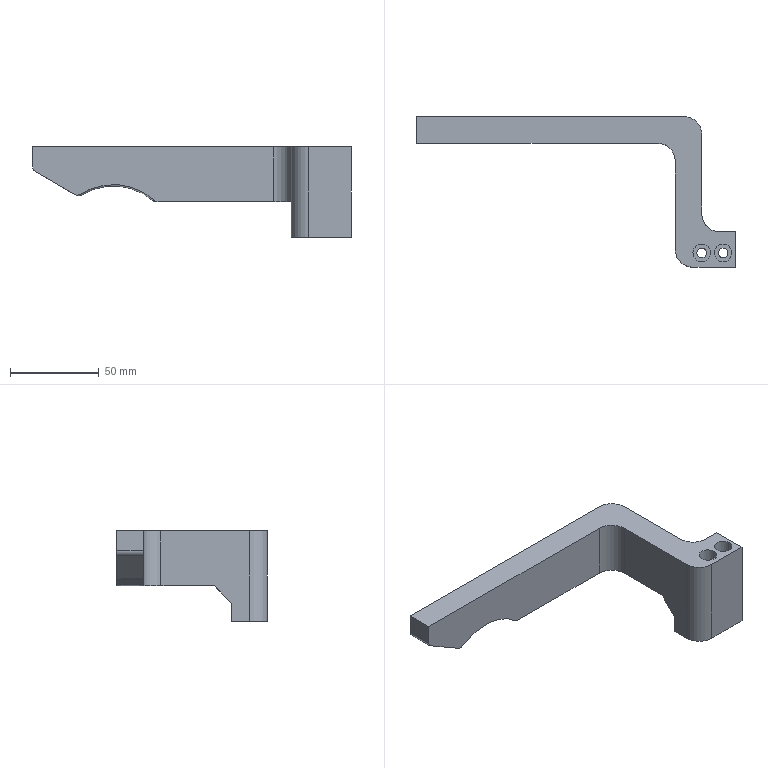NC program | NX | posted with a generic post | part box 180 x 85 x 51 mm
Lines 27156 to 29209 of 44959, first 1814 of 2034 lines:
(FLOOR_WALL_COPY , TOOL : D63)
N54298 T01 M6
N54300 G54
N54302 G17 G0 G90 X-129.5 Y-19. S6500 M3
N54304 G43 Z30. H1
N54306 Z3.
N54308 G94 G1 Z0. F1500.
N54310 X-121.503
N54312 X102.503
N54314 X105.503
N54316 Z3.
N54318 G0 Z30.
N54320 X-129.5
N54322 Z2.
N54324 G1 Z-1.
N54326 X-121.503
N54328 X102.503
N54330 X105.503
N54332 Z2.
N54334 G0 Z30.
N54336 X-129.5
N54338 Z1.
N54340 G1 Z-2.
N54342 X-121.503
N54344 X102.503
N54346 X105.503
N54348 Z1.
N54350 G0 Z30.
N54352 X-129.5
N54354 Z0.
N54356 G1 Z-3.
N54358 X-121.503
N54360 X102.503
N54362 X105.503
N54364 Z0.
N54366 G0 Z30.
N54368 X-129.5
N54370 Z-1.
N54372 G1 Z-4.
N54374 X-121.503
N54376 X102.503
N54378 X105.503
N54380 Z-1.
N54382 G0 Z30.
N54384 X-129.5
N54386 Z-2.
N54388 G1 Z-5.
N54390 X-121.503
N54392 X102.503
N54394 X105.503
N54396 Z-2.
N54398 G0 Z30.
N54400 X-129.5
N54402 Z-3.
N54404 G1 Z-6.
N54406 X-121.503
N54408 X102.503
N54410 X105.503
N54412 Z-3.
N54414 G0 Z30.
N54416 X-129.5
N54418 Z-4.
N54420 G1 Z-7.
N54422 X-121.503
N54424 X102.503
N54426 X105.503
N54428 Z-4.
N54430 G0 Z30.
N54432 X-129.5
N54434 Z-5.
N54436 G1 Z-8.
N54438 X-121.503
N54440 X102.503
N54442 X105.503
N54444 Z-5.
N54446 G0 Z30.
N54448 X-129.5
N54450 Z-6.
N54452 G1 Z-9.
N54454 X-121.503
N54456 X102.503
N54458 X105.503
N54460 Z-6.
N54462 G0 Z30.
N54464 X-129.5
N54466 Z-7.
N54468 G1 Z-10.
N54470 X-121.503
N54472 X102.503
N54474 X105.503
N54476 Z-7.
N54478 G0 Z30.
N54480 X-129.5
N54482 Z-8.
N54484 G1 Z-11.
N54486 X-121.503
N54488 X102.503
N54490 X105.503
N54492 Z-8.
N54494 G0 Z30.
N54496 X-129.5
N54498 Z-9.
N54500 G1 Z-12.
N54502 X-121.503
N54504 X102.503
N54506 X105.503
N54508 Z-9.
N54510 G0 Z30.
N54512 X-129.5
N54514 Z-10.
N54516 G1 Z-13.
N54518 X-121.503
N54520 X102.503
N54522 X105.503
N54524 Z-10.
N54526 G0 Z30.
N54528 X-129.5
N54530 Z-11.
N54532 G1 Z-14.
N54534 X-121.503
N54536 X102.503
N54538 X105.503
N54540 Z-11.
N54542 G0 Z30.
N54544 X-129.5
N54546 Z-12.
N54548 G1 Z-15.
N54550 X-121.503
N54552 X102.503
N54554 X105.503
N54556 Z-12.
N54558 G0 Z30.
N54560 X-129.5
N54562 Z-13.
N54564 G1 Z-16.
N54566 X-121.503
N54568 X102.503
N54570 X105.503
N54572 Z-13.
N54574 G0 Z30.
N54576 X-129.5
N54578 Z-14.
N54580 G1 Z-17.
N54582 X-121.503
N54584 X102.503
N54586 X105.503
N54588 Z-14.
N54590 G0 Z30.
N54592 X-129.5
N54594 Z-15.
N54596 G1 Z-18.
N54598 X-121.503
N54600 X102.503
N54602 X105.503
N54604 Z-15.
N54606 G0 Z30.
N54608 X-129.5
N54610 Z-16.
N54612 G1 Z-19.
N54614 X-121.503
N54616 X102.503
N54618 X105.503
N54620 Z-16.
N54622 G0 Z30.
N54624 X-129.5
N54626 Z-17.
N54628 G1 Z-20.
N54630 X-121.503
N54632 X102.503
N54634 X105.503
N54636 Z-17.
N54638 G0 Z30.
N54640 M5
(ZLEVEL_PROFILE , TOOL : D12C)
N54642 T12 M6
N54644 G54
N54646 G17 G0 G90 X98.933 Y13.081 S9500 M3
N54648 G43 Z30. H12
N54650 Z2.51
N54652 G94 G1 Z-0.49 F1000.
N54654 X97.362 Y15.801
N54656 G3 X96.323 Y16.401 R1.2
N54658 G1 X85.881 Y16.4 F2500.
N54660 X56.
N54662 X55.197 Y16.453
N54664 X55.137 Y16.4
N54666 X49.677 Y16.401
N54668 Z-0.98
N54670 X55.137 Y16.4
N54672 X55.197 Y16.453
N54674 X56. Y16.4
N54676 X85.881
N54678 X96.323 Y16.401
N54680 Z-1.47
N54682 X85.881 Y16.4
N54684 X56.
N54686 X55.197 Y16.453
N54688 X55.137 Y16.4
N54690 X49.677
N54692 Z-1.96
N54694 X55.137
N54696 X55.197 Y16.453
N54698 X56. Y16.4
N54700 X85.881
N54702 X96.323 Y16.401
N54704 Z-2.45
N54706 X85.881 Y16.4
N54708 X56.
N54710 X55.197 Y16.453
N54712 X55.137 Y16.4
N54714 X49.677
N54716 Z-2.94
N54718 X55.137
N54720 X55.197 Y16.453
N54722 X56. Y16.4
N54724 X85.881
N54726 X96.323 Y16.401
N54728 Z-3.43
N54730 X85.881 Y16.4
N54732 X56.
N54734 X55.197 Y16.453
N54736 X55.137 Y16.4
N54738 X49.677
N54740 Z-3.92
N54742 X55.137
N54744 X55.197 Y16.453
N54746 X56. Y16.4
N54748 X85.881
N54750 X96.323 Y16.401
N54752 Z-4.41
N54754 X85.881 Y16.4
N54756 X56.462
N54758 G2 X55.197 Y16.453 R9.583
N54760 G1 X55.137 Y16.4
N54762 X49.677
N54764 Z-4.9
N54766 X55.137
N54768 X55.197 Y16.453
N54770 G3 X56.462 Y16.4 R9.572
N54772 G1 X85.881
N54774 X96.323 Y16.401
N54776 Z-5.39
N54778 X85.881 Y16.4
N54780 X56.462
N54782 G2 X55.197 Y16.453 R9.562
N54784 G1 X55.137 Y16.4
N54786 X49.677
N54788 Z-5.88
N54790 X55.137
N54792 X55.197 Y16.453
N54794 G3 X56.462 Y16.4 R9.551
N54796 G1 X85.881
N54798 X96.323 Y16.401
N54800 Z-6.37
N54802 X85.881 Y16.4
N54804 X56.462
N54806 G2 X55.197 Y16.453 R9.54
N54808 G1 X55.137 Y16.4
N54810 X49.677
N54812 Z-6.86
N54814 X55.137
N54816 X55.197 Y16.453
N54818 G3 X56.462 Y16.4 R9.529
N54820 G1 X85.881
N54822 X96.323 Y16.401
N54824 Z-7.35
N54826 X85.881 Y16.4
N54828 X56.462
N54830 G2 X55.197 Y16.453 R9.518
N54832 G1 X55.137 Y16.4
N54834 X49.677
N54836 Z-7.84
N54838 X55.137
N54840 X55.197 Y16.453
N54842 G3 X56.462 Y16.4 R9.507
N54844 G1 X85.881
N54846 X96.323 Y16.401
N54848 Z-8.33
N54850 X85.881 Y16.4
N54852 X56.462
N54854 G2 X55.197 Y16.453 R9.497
N54856 G1 X55.137 Y16.4
N54858 X49.677
N54860 Z-8.82
N54862 X55.137
N54864 X55.197 Y16.453
N54866 G3 X56.462 Y16.4 R9.486
N54868 G1 X85.881
N54870 X96.323 Y16.401
N54872 Z-9.31
N54874 X85.881 Y16.4
N54876 X56.462
N54878 G2 X55.197 Y16.453 R9.475
N54880 G1 X55.137 Y16.4
N54882 X49.677
N54884 Z-9.8
N54886 X55.137
N54888 X55.197 Y16.453
N54890 G3 X56.462 Y16.4 R9.465
N54892 G1 X85.881
N54894 X96.323 Y16.401
N54896 G2 X97.362 Y15.801 R1.2
N54898 G1 X98.933 Y13.081
N54900 Z-6.8
N54902 G0 Z30.
(ZLEVEL_PROFILE_COPY , TOOL : D12C)
N54904 X87.319 Y12.8
N54906 Z-7.495
N54908 G1 Z-10.495 F1000.
N54910 X85.147 Y15.894
N54912 G3 X84.059 Y16.4 R1.2
N54914 X82.377 Y16.013 R6.277 F2500.
N54916 G1 X81.536 Y15.884
N54918 X77.7 Y15.864
N54920 X49.577
N54922 X49.512 Y15.867
N54924 X49.51 Y15.616 Z-10.743
N54926 X49.509 Y15.372 Z-10.99
N54928 X56. Y15.369
N54930 X81.101
N54932 G3 X84.182 Y16.235 R5.914
N54934 G1 X84.9 Y16.4
N54936 X85.741 Z-11.485
N54938 X84.937 Y16.235
N54940 G2 X81.271 Y14.884 R5.938
N54942 G1 X80.695 Y14.874
N54944 X49.577
N54946 X49.507 Y14.878
N54948 X49.506 Y14.626 Z-11.733
N54950 X49.504 Y14.383 Z-11.98
N54952 X49.577 Y14.379
N54954 X81.208
N54956 G3 X85.228 Y15.974 R5.862
N54958 G1 X85.505 Y16.235
N54960 X85.741 Y16.4
N54962 X86.582 Z-12.475
N54964 X86.023 Y16.235
N54966 G2 X81.312 Y13.889 R6.015
N54968 G1 X80.695 Y13.884
N54970 X49.577
N54972 X49.502 Y13.888
N54974 X49.501 Y13.636 Z-12.723
N54976 X49.5 Y13.393 Z-12.97
N54978 X49.577 Y13.389
N54980 X80.695
N54982 X81.317 Y13.392
N54984 G3 X86.582 Y16.4 R6.167
N54986 G1 X87.423 Z-13.465
N54988 X86.818 Y16.235
N54990 G2 X81.536 Y12.895 R6.072
N54992 G1 X73.375 Y12.894
N54994 X49.577
N54996 X49.498 Y12.898
N54998 Y12.646 Z-13.713
N55000 Y12.403 Z-13.96
N55002 X49.577 Y12.399
N55004 X72.978
N55006 X81.536
N55008 G3 X87.128 Y16.235 R6.086
N55010 G1 X87.423 Y16.4
N55012 X88.264 Z-14.455
N55014 X87.423 Y16.302
N55016 G2 X81.536 Y11.904 R6.089
N55018 G1 X49.577
N55020 X49.498 Y11.908
N55022 Y11.656 Z-14.703
N55024 Y11.413 Z-14.95
N55026 X49.577 Y11.409
N55028 X79.854
N55030 X80.302 Y11.422
N55032 X79.966 Y11.163 Z-15.198
N55034 X79.629 Y10.925 Z-15.445
N55036 X79.013 Y10.914
N55038 X49.577
N55040 X49.498 Y10.918
N55042 Y10.666 Z-15.693
N55044 Y10.423 Z-15.94
N55046 X49.577 Y10.419
N55048 X71.835
N55050 X79.139 Y10.426
N55052 X78.96 Y10.171 Z-16.188
N55054 X78.78 Y9.931 Z-16.435
N55056 X78.172 Y9.924
N55058 X49.577
N55060 X49.498 Y9.928
N55062 X49.499 Y9.676 Z-16.683
N55064 Y9.433 Z-16.93
N55066 X49.577 Y9.429
N55068 X78.172
N55070 X78.469 Y9.437
N55072 X78.356 Y9.181 Z-17.178
N55074 X78.243 Y8.938 Z-17.425
N55076 X78.172 Y8.934
N55078 X49.577
N55080 X49.502 Y8.938
N55082 X49.503 Y8.686 Z-17.673
N55084 X49.505 Y8.443 Z-17.92
N55086 X49.577 Y8.439
N55088 X71.208
N55090 X78.063 Y8.44
N55092 X77.991 Y8.191 Z-18.168
N55094 X77.92 Y7.948 Z-18.415
N55096 X71.444 Y7.944
N55098 X49.577
N55100 X49.507 Y7.948
N55102 X49.508 Y7.696 Z-18.663
N55104 X49.509 Y7.453 Z-18.91
N55106 X49.577 Y7.449
N55108 X71.058
N55110 X77.822 Y7.455
N55112 X77.782 Y7.201 Z-19.158
N55114 X77.743 Y6.956 Z-19.405
N55116 X71.019 Y6.954
N55118 X56.
N55120 X49.512 Y6.955
N55122 X49.513 Y6.706 Z-19.653
N55124 X49.514 Y6.47 Z-19.9
N55126 X56. Y6.466
N55128 X77.331
N55130 X77.691 Y6.474
N55132 G2 X78.744 Y5.898 R1.2
N55134 G1 X80.35 Y3.257
N55136 Z-16.9
N55138 G0 Z30.
(ZLEVEL_PROFILE_COPY_COPY_COPY , TOOL : D12C)
N55140 X-69.287 Y-51.578
N55142 Z-17.491
N55144 G1 Z-20.491 F1000.
N55146 X-66.638 Y-50.047
N55148 G3 X-66.039 Y-49.008 R1.2
N55150 G1 X-66.045 Y-37.949 F2500.
N55152 X-66.03 Y-37.719
N55154 G3 X-66.563 Y-36.644 R1.2
N55156 G1 X-69.324 Y-34.809
N55158 Z-17.491
N55160 G0 X-70.204 Y-19.451 Z-17.982
N55162 G1 Z-20.982 F1000.
N55164 X-67.458 Y-21.119
N55166 G2 X-66.881 Y-22.171 R1.2
N55168 G1 X-66.895 Y-22.783 F2500.
N55170 X-66.889 Y-49.013
N55172 X-67.32 Y-49.015 Z-21.227
N55174 X-67.739 Y-49.018 Z-21.472
N55176 Y-20.995
N55178 X-68.17 Y-20.992 Z-21.718
N55180 X-68.589 Y-20.99 Z-21.963
N55182 Y-49.023
N55184 X-69.02 Y-49.025 Z-22.209
N55186 X-69.439 Y-49.028 Z-22.454
N55188 Y-20.984
N55190 X-69.87 Y-20.981 Z-22.7
N55192 X-70.289 Y-20.979 Z-22.945
N55194 X-70.295 Y-21.098
N55196 X-70.289 Y-49.033
N55198 X-70.72 Y-49.035 Z-23.19
N55200 X-71.139 Y-49.038 Z-23.436
N55202 X-71.145 Y-48.902
N55204 X-71.139 Y-20.973
N55206 X-71.57 Y-20.97 Z-23.681
N55208 X-71.989 Y-20.967 Z-23.927
N55210 X-71.996 Y-32.744
N55212 Y-42.5
N55214 Y-48.902
N55216 X-71.989 Y-49.042
N55218 X-72.421 Y-49.045 Z-24.172
N55220 X-72.839 Y-49.047 Z-24.417
N55222 X-72.846 Y-48.902
N55224 Y-42.5
N55226 Y-27.5
N55228 Y-21.098
N55230 X-72.839 Y-20.962
N55232 X-73.271 Y-20.959 Z-24.663
N55234 X-73.689 Y-20.956 Z-24.908
N55236 X-73.696 Y-21.098
N55238 Y-27.5
N55240 Y-42.5
N55242 Y-48.902
N55244 X-73.689 Y-49.052
N55246 X-74.121 Y-49.055 Z-25.154
N55248 X-74.539 Y-49.057 Z-25.399
N55250 X-74.546 Y-48.902
N55252 Y-42.5
N55254 Y-27.5
N55256 Y-21.098
N55258 X-74.539 Y-20.951
N55260 X-74.971 Y-20.948 Z-25.645
N55262 X-75.389 Y-20.945 Z-25.89
N55264 X-75.396 Y-21.098
N55266 Y-27.5
N55268 Y-42.5
N55270 Y-48.902
N55272 X-75.389 Y-49.062
N55274 X-75.821 Y-49.064 Z-26.135
N55276 X-76.239 Y-49.067 Z-26.381
N55278 X-76.246 Y-48.902
N55280 Y-42.5
N55282 Y-27.5
N55284 Y-21.098
N55286 X-76.239 Y-20.94
N55288 X-76.671 Y-20.937 Z-26.626
N55290 X-77.089 Y-20.935 Z-26.872
N55292 X-77.096 Y-21.098
N55294 Y-27.5
N55296 Y-42.5
N55298 Y-48.902
N55300 X-77.089 Y-49.07
N55302 X-77.521 Y-49.072 Z-27.117
N55304 X-77.939 Y-49.074 Z-27.362
N55306 X-77.946 Y-48.902
N55308 X-77.947 Y-42.5
N55310 Y-27.5
N55312 X-77.946 Y-21.098
N55314 X-77.939 Y-20.931
N55316 X-78.371 Y-20.929 Z-27.608
N55318 X-78.788 Y-20.927 Z-27.853
N55320 X-78.796 Y-21.098
N55322 X-78.797 Y-27.5
N55324 Y-42.5
N55326 X-78.796 Y-48.902
N55328 X-78.789 Y-49.078
N55330 X-79.221 Y-49.079 Z-28.099
N55332 X-79.639 Y-49.081 Z-28.344
N55334 X-79.647 Y-48.902
N55336 Y-42.5
N55338 Y-27.5
N55340 X-79.646 Y-21.098
N55342 X-79.638 Y-20.923
N55344 X-80.071 Y-20.921 Z-28.589
N55346 X-80.488 Y-20.919 Z-28.835
N55348 X-80.496 Y-21.098
N55350 X-80.497 Y-27.5
N55352 Y-42.5
N55354 Y-48.902
N55356 X-80.489 Y-49.085
N55358 X-80.921 Y-49.086 Z-29.08
N55360 X-81.338 Y-49.087 Z-29.326
N55362 X-81.346 Y-48.902
N55364 X-81.347 Y-42.5
N55366 Y-27.5
N55368 X-81.345 Y-21.098
N55370 X-81.338 Y-20.915
N55372 X-81.769 Y-20.914 Z-29.571
N55374 X-82.186 Y-20.913 Z-29.817
N55376 X-82.194 Y-21.098
N55378 X-82.197 Y-27.5
N55380 Y-42.5
N55382 X-82.196 Y-48.902
N55384 X-82.188 Y-49.089
N55386 X-82.62 Z-30.062
N55388 X-83.037 Y-49.09 Z-30.307
N55390 X-83.045 Y-48.902
N55392 X-83.047 Y-42.5
N55394 Y-27.5
N55396 X-83.042 Y-21.098
N55398 X-83.034 Y-20.911
N55400 X-83.465 Y-20.91 Z-30.553
N55402 X-83.882 Y-20.909 Z-30.798
N55404 X-83.89 Y-21.098
N55406 X-83.898 Y-27.5
N55408 Y-42.5
N55410 X-83.894 Y-48.902
N55412 X-83.886 Y-49.092
N55414 X-84.319 Y-49.093 Z-31.044
N55416 X-84.736 Y-49.094 Z-31.289
N55418 X-84.744 Y-48.902
N55420 X-84.748 Y-42.5
N55422 Y-27.5
N55424 X-84.738 Y-21.098
N55426 X-84.73 Y-20.907
N55428 X-85.161 Y-20.906 Z-31.534
N55430 X-85.576 Z-31.78
N55432 X-85.585 Y-21.098
N55434 X-85.598 Y-27.5
N55436 Y-42.5
N55438 X-85.591 Y-48.902
N55440 X-85.583 Y-49.095
N55442 X-86.013 Z-32.025
N55444 X-86.427 Y-49.096 Z-32.271
N55446 X-86.448 Y-42.5
N55448 Y-27.5
N55450 X-86.426 Y-21.098
N55452 X-86.417 Y-20.905
N55454 X-86.842 Y-20.904 Z-32.516
N55456 X-87.254 Z-32.762
N55458 X-87.274 Y-21.941
N55460 X-87.298 Y-27.5
N55462 Y-42.5
N55464 X-87.291 Y-43.004
N55466 X-87.27 Y-49.097
N55468 X-87.7 Z-33.007
N55470 X-88.114 Z-33.252
N55472 X-88.148 Y-42.5
N55474 Y-27.5
N55476 X-88.112 Y-21.941
N55478 X-88.091 Y-20.903
N55480 X-88.516 Z-33.498
N55482 X-88.928 Y-20.902 Z-33.743
N55484 X-88.937 Y-21.098
N55486 X-88.998 Y-26.996
N55488 Y-27.5
N55490 Y-42.5
N55492 X-88.957 Y-49.098
N55494 X-89.387 Z-33.989
N55496 X-89.795 Z-34.234
N55498 X-89.836 Y-43.004
N55500 X-89.848 Y-42.5
N55502 Y-27.5
N55504 X-89.772 Y-21.098
N55506 X-89.763 Y-20.902
N55508 X-90.184 Z-34.479
N55510 X-90.59 Z-34.725
N55512 X-90.699 Y-27.5
N55514 Y-42.5
N55516 X-90.619 Y-49.099
N55518 X-91.035 Z-34.97
N55520 X-91.433 Z-35.216
N55522 G3 X-91.549 Y-42.5 R99.552
N55524 G1 Y-27.5
N55526 X-91.41 Y-20.901
N55528 X-91.829 Z-35.461
N55530 X-92.231 Z-35.706
N55532 X-92.399 Y-27.5
N55534 Y-42.5
N55536 G2 X-92.248 Y-49.099 R80.604
N55538 G1 X-92.664 Z-35.952
N55540 X-93.063 Z-36.197
N55542 G3 X-93.249 Y-42.5 R68.833
N55544 G1 Y-27.5
N55546 G3 X-93.052 Y-20.901 R129.699
N55548 G1 X-93.471 Z-36.443
N55550 X-93.869 Z-36.688
N55552 G2 X-94.099 Y-27.5 R74.476
N55554 G1 Y-42.5
N55556 G2 X-93.873 Y-49.099 R63.359
N55558 G1 X-94.293 Y-49.1 Z-36.934
N55560 X-94.648 Z-37.179
N55562 G3 X-94.894 Y-42.5 R56.988
N55564 G1 Y-27.5
N55566 G3 X-94.648 Y-20.9 R56.988
N55568 G1 X-94.816 Z-37.302
N55570 X-94.964 Y-20.899 Z-37.424
N55572 X-95.113 Z-37.547
N55574 X-95.188 Z-37.67
N55576 G2 X-95.399 Y-27.5 R70.632
N55578 G1 Y-42.5
N55580 G2 X-95.188 Y-49.101 R70.632
N55582 G1 X-95.39 Y-49.105 Z-37.915
N55584 X-95.577 Y-49.109 Z-38.161
N55586 G3 X-95.728 Y-42.5 R101.347
N55588 G1 Y-27.5
N55590 G3 X-95.578 Y-20.892 R98.089
N55592 G1 X-95.691 Y-20.888 Z-38.406
N55594 X-95.8 Y-20.885 Z-38.651
N55596 G2 X-95.94 Y-27.5 R102.606
N55598 G1 Y-42.5
N55600 G2 X-95.787 Y-49.115 R131.912
N55602 G1 X-95.885 Y-49.118 Z-38.897
N55604 X-95.963 Y-49.122 Z-39.142
N55606 G3 X-96.061 Y-42.5 R267.017
N55608 G1 Y-27.5
N55610 G3 X-95.972 Y-20.879 R163.327
N55612 G1 X-96.042 Y-20.877 Z-39.388
N55614 X-96.087 Z-39.633
N55616 X-96.095 Y-21.098
N55618 Y-48.902
N55620 X-96.087 Y-49.123
N55622 G2 X-96.65 Y-50.183 R1.2
N55624 G1 X-99.302 Y-51.843
N55626 Z-36.633
N55628 G0 Z30.
(ZLEVEL_PROFILE_COPY_COPY , TOOL : D12C)
N55630 X-59.223 Y-29.939
N55632 Z-17.485
N55634 G1 Z-20.485 F1000.
N55636 X-61.809 Y-31.789
N55638 G3 X-62.305 Y-32.882 R1.2
N55640 G1 X-60.794 Y-48.32 F2500.
N55642 X-60.381 Y-48.33 Z-20.728
N55644 X-59.992 Y-48.34 Z-20.971
N55646 X-60.12 Y-47.217
N55648 X-62.666 Y-20.651
N55650 X-62.283 Y-20.553 Z-21.214
N55652 X-61.907 Y-20.458 Z-21.456
N55654 X-59.784 Y-43.004
N55656 X-59.19 Y-48.36
N55658 X-58.777 Y-48.369 Z-21.699
N55660 X-58.379 Y-48.379 Z-21.942
N55662 X-58.825 Y-44.689
N55664 X-61.129 Y-20.449
N55666 X-60.738 Y-20.444 Z-22.185
N55668 X-60.351 Y-20.439 Z-22.427
N55670 X-58.131 Y-43.846
N55672 X-57.586 Y-48.399
N55674 X-57.173 Y-48.409 Z-22.67
N55676 X-56.784 Y-48.419 Z-22.913
N55678 G2 X-59.573 Y-20.43 R774.757
N55680 G1 X-59.185 Y-20.425 Z-23.156
N55682 X-58.795 Y-20.42 Z-23.398
N55684 G3 X-56.767 Y-42.161 R1335.362
N55686 G1 X-56.645 Y-43.004
N55688 X-55.992 Y-48.059
N55690 X-55.962 Y-48.428
N55692 X-55.526 Y-48.422 Z-23.641
N55694 X-55.105 Y-48.417 Z-23.884
N55696 X-56.048 Y-41.319
N55698 G2 X-58.017 Y-20.411 R1461.229
N55700 G1 X-57.631 Y-20.403 Z-24.126
N55702 X-57.218 Y-20.395 Z-24.369
N55704 G2 X-56.693 Y-26.368 R55.634
N55706 G1 X-56.672 Y-26.996
N55708 X-56.605 Y-27.839
N55710 X-55.216 Y-41.319
N55712 X-55.104 Y-42.161
N55714 G2 X-54.229 Y-48.399 R53.906
N55716 G1 X-53.731 Y-48.382 Z-24.612
N55718 X-53.242 Y-48.365 Z-24.855
N55720 G3 X-54.335 Y-41.319 R57.54
N55722 G1 X-55.604 Y-29.524
N55724 X-55.777 Y-27.839
N55726 G3 X-56.375 Y-20.365 R68.173
N55728 G1 X-55.942 Y-20.346 Z-25.097
N55730 X-55.513 Y-20.327 Z-25.34
N55732 G2 X-55.003 Y-27.131 R49.02
N55734 G1 X-53.355 Y-41.319
N55736 G2 X-52.238 Y-48.326 R49.439
N55738 G1 X-51.718 Y-48.299 Z-25.583
N55740 X-51.114 Y-48.267 Z-25.826
N55742 G3 X-52.342 Y-41.319 R44.347
N55744 G1 X-52.469 Y-40.373
N55746 X-53.972 Y-27.839
N55748 X-54.055 Y-26.996
N55750 G3 X-54.599 Y-20.284 R40.878
N55752 G1 X-54.105 Y-20.259 Z-26.068
N55754 X-53.61 Y-20.234 Z-26.311
N55756 G2 X-53.055 Y-26.996 R32.758
N55758 G1 X-52.972 Y-27.839
N55760 X-51.178 Y-41.319
N55762 G2 X-49.867 Y-48.185 R29.497
N55764 G3 X-49.196 Y-49.18 R1.2
N55766 G1 X-46.323 Y-50.581
N55768 Z-23.311
N55770 G0 Z30.
N55772 X-32.005 Y-50.939
N55774 Z-17.485
N55776 G1 Z-20.485 F1000.
N55778 X-29.243 Y-49.6
N55780 G3 X-28.569 Y-48.607 R1.2
N55782 G2 X-26.34 Y-20.43 R2133.304 F2500.
N55784 G1 X-26.701 Y-20.431 Z-20.728
N55786 X-27.029 Z-20.971
N55788 X-27.127 Y-21.941
N55790 X-29.241 Y-48.059
N55792 X-29.27 Y-48.597
N55794 X-29.616 Y-48.589 Z-21.214
N55796 X-29.967 Y-48.581 Z-21.456
N55798 G3 X-27.662 Y-20.423 R1113.98
N55800 G1 X-27.975 Y-20.419 Z-21.699
N55802 X-28.284 Y-20.415 Z-21.942
N55804 G3 X-28.684 Y-26.996 R111.738
N55806 G1 X-29.895 Y-41.319
N55808 G3 X-30.682 Y-48.565 R76.199
N55810 G1 X-31.045 Y-48.557 Z-22.185
N55812 X-31.402 Y-48.549 Z-22.427
N55814 G2 X-30.58 Y-41.319 R68.15
N55816 G1 X-29.523 Y-29.524
N55818 X-29.317 Y-26.996
N55820 G2 X-28.911 Y-20.405 R72.504
N55822 G1 X-29.234 Y-20.399 Z-22.67
N55824 X-29.577 Y-20.392 Z-22.913
N55826 G3 X-29.981 Y-26.996 R63.39
N55828 G1 X-30.044 Y-27.839
N55830 X-31.264 Y-41.319
N55832 G3 X-32.121 Y-48.532 R63.417
N55834 G1 X-32.527 Y-48.52 Z-23.156
N55836 X-32.929 Y-48.507 Z-23.398
N55838 G2 X-31.985 Y-41.319 R58.139
N55840 G1 X-30.729 Y-27.839
N55842 X-30.667 Y-26.996
N55844 G2 X-30.258 Y-20.378 R57.242
N55846 G1 X-30.601 Y-20.371 Z-23.641
N55848 X-30.941 Y-20.364 Z-23.884
N55850 G3 X-31.357 Y-26.996 R46.023
N55852 G1 X-32.778 Y-41.319
N55854 G3 X-33.747 Y-48.481 R50.008
N55856 G1 X-34.163 Y-48.466 Z-24.126
N55858 X-34.594 Y-48.451 Z-24.369
N55860 G2 X-33.598 Y-41.319 R52.623
N55862 G1 X-32.213 Y-27.839
N55864 X-32.148 Y-26.996
N55866 G2 X-31.677 Y-20.345 R47.282
N55868 G1 X-32.083 Y-20.332 Z-24.612
N55870 X-32.492 Y-20.319 Z-24.855
N55872 G3 X-32.967 Y-26.996 R40.96
N55874 G1 X-34.473 Y-41.319
N55876 G3 X-35.574 Y-48.406 R47.365
N55878 G1 X-36.072 Y-48.382 Z-25.097
N55880 X-36.571 Y-48.358 Z-25.34
N55882 G2 X-35.445 Y-41.319 R44.741
N55884 G1 X-33.853 Y-27.839
N55886 G2 X-33.312 Y-20.293 R68.026
N55888 G1 X-33.717 Y-20.278 Z-25.583
N55890 X-34.19 Y-20.26 Z-25.826
N55892 G3 X-34.745 Y-26.996 R39.476
N55894 G1 X-34.829 Y-27.839
N55896 X-36.417 Y-41.093
N55898 G3 X-37.695 Y-48.289 R48.673
N55900 G1 X-38.324 Y-48.245 Z-26.068
N55902 X-38.941 Y-48.201 Z-26.311
N55904 G2 X-37.623 Y-41.319 R28.912
N55906 G1 X-37.486 Y-40.476
N55908 X-35.828 Y-27.839
N55910 X-35.744 Y-26.996
N55912 G2 X-35.181 Y-20.216 R32.726
N55914 G1 X-35.68 Y-20.193 Z-26.554
N55916 X-36.176 Y-20.17 Z-26.797
N55918 G3 X-36.812 Y-26.996 R41.658
N55920 G1 X-36.917 Y-27.839
N55922 X-38.737 Y-40.476
N55924 X-38.874 Y-41.319
N55926 G3 X-40.377 Y-48.062 R38.627
N55928 G2 X-41.106 Y-49.015 R1.2
N55930 G1 X-43.997 Y-50.216
N55932 Z-23.797
N55934 G0 Z30.
N55936 X-49.815 Y-17.009
N55938 Z-23.797
N55940 G1 Z-26.797 F1000.
N55942 X-52.217 Y-19.053
N55944 G3 X-52.619 Y-20.183 R1.2
N55946 G2 X-51.982 Y-26.996 R38.789 F2500.
N55948 G1 X-51.879 Y-27.839
N55950 X-49.934 Y-41.265
N55952 G2 X-48.433 Y-48.053 R39.921
N55954 G1 X-47.63 Y-47.957 Z-27.039
N55956 X-46.806 Y-47.859 Z-27.282
N55958 G3 X-48.615 Y-40.476 R39.323
N55960 G1 X-50.641 Y-27.839
N55962 X-50.752 Y-26.996
N55964 G3 X-51.437 Y-20.105 R27.027
N55966 G2 X-51.086 Y-18.957 R1.2
N55968 G1 X-48.74 Y-16.766
N55970 Z-24.282
N55972 G0 Z30.
N55974 X-44.41 Y-53.982
N55976 Z-24.282
N55978 G1 Z-27.282 F1000.
N55980 X-42.765 Y-48.794
N55982 G3 X-42.015 Y-47.857 R1.2
N55984 G2 X-40.186 Y-40.476 R41.614 F2500.
N55986 G1 X-39.796 Y-38.364
N55988 X-38.047 Y-26.996
N55990 G2 X-37.356 Y-20.096 R31.644
N55992 G1 X-37.982 Y-20.054 Z-27.525
N55994 X-38.591 Y-20.013 Z-27.767
N55996 G3 X-39.373 Y-26.996 R35.852
N55998 G1 X-39.514 Y-27.839
N56000 X-41.486 Y-38.636
N56002 X-41.887 Y-40.476
N56004 G3 X-44.186 Y-47.638 R27.782
N56006 G1 Z-24.767
N56008 G0 Z30.
N56010 X-47.487 Y-16.75
N56012 Z-24.767
N56014 G1 Z-27.767 F1000.
N56016 X-49.833 Y-18.876
N56018 G3 X-50.201 Y-20.018 R1.2
N56020 G2 X-49.424 Y-26.996 R34.641 F2500.
N56022 G1 X-49.089 Y-29.016
N56024 X-47.1 Y-39.634
N56026 X-46.915 Y-40.476
N56028 G2 X-44.619 Y-47.638 R27.792
N56030 G1 Z-24.767
N56032 G0 X-42.84 Y-16.816 Z-25.253
N56034 G1 Z-28.253 F1000.
N56036 X-40.492 Y-18.745
N56038 G2 X-40.071 Y-19.868 R1.2
N56040 G1 X-40.973 Y-25.311 F2500.
N56042 X-40.972 Y-26.154
N56044 G2 X-44.02 Y-40.036 R75.549
N56046 G1 X-44.395 Y-40.642
N56048 X-44.865 Y-39.821
N56050 X-44.924 Y-39.634
N56052 X-47.4 Y-29.276
N56054 X-47.821 Y-26.996
N56056 G3 X-48.721 Y-19.871 R26.33
N56058 G1 X-47.912 Y-19.771 Z-28.496
N56060 X-47.059 Y-19.664 Z-28.738
N56062 G2 X-45.839 Y-26.996 R28.251
N56064 G1 X-44.405 Y-32.581
N56066 G3 X-42.852 Y-24.469 R21.836
N56068 G1 X-41.722 Y-19.669
N56070 X-42.77 Y-19.454 Z-28.981
N56072 X-43.862 Y-19.23 Z-29.224
N56074 X-44.403 Y-21.219
N56076 X-44.931 Y-19.228
N56078 G2 X-44.617 Y-18.07 R1.2
N56080 G1 X-44.4 Y-13.672
N56082 Z-26.224
N56084 G0 Z30.
N56086 M5
(ZLEVEL_PROFILE_COPY_COPY_COPY_1 , TOOL : D10)
N56088 T10 M6
N56090 G54
N56092 G17 G0 G90 X100.829 Y34.4 S9500 M3
N56094 G43 Z30. H10
N56096 Z-0.487
N56098 G94 G1 X96.151 Y34.904 F1000.
N56100 G3 X95.283 Y35.401 R1.
N56102 G1 X94.509 Y35.399 F2500.
N56104 X89.089 Y35.4
N56106 X64.
N56108 G3 X63. Y34.4 R1.
N56110 X64. Y33.4 R1.
N56112 G1 X89.089
N56114 X94.509 Y33.401
N56116 X95.283 Y33.399
N56118 G3 X96.151 Y33.896 R1.
N56120 G1 X100.829 Y34.4
N56122 G0 Z-0.974
N56124 G1 X96.151 Y34.904 F1000.
N56126 G3 X95.283 Y35.401 R1.
N56128 G1 X94.509 Y35.399 F2500.
N56130 X89.089 Y35.4
N56132 X64.
N56134 G3 X63. Y34.4 R1.
N56136 X64. Y33.4 R1.
N56138 G1 X89.089
N56140 X94.509 Y33.401
N56142 X95.283 Y33.399
N56144 G3 X96.151 Y33.896 R1.
N56146 G1 X100.829 Y34.4
N56148 G0 Z-1.461
N56150 G1 X96.151 Y34.904 F1000.
N56152 G3 X95.283 Y35.401 R1.
N56154 G1 X94.509 Y35.398 F2500.
N56156 X89.089 Y35.4
N56158 X64.
N56160 G3 X63. Y34.4 R1.
N56162 X64. Y33.4 R1.
N56164 G1 X89.089
N56166 X94.509 Y33.402
N56168 X95.283 Y33.399
N56170 G3 X96.151 Y33.896 R1.
N56172 G1 X100.829 Y34.4
N56174 G0 Z-1.948
N56176 G1 X96.151 Y34.904 F1000.
N56178 G3 X95.283 Y35.401 R1.
N56180 G1 X94.509 Y35.398 F2500.
N56182 X89.089 Y35.4
N56184 X64.
N56186 G3 X63. Y34.4 R1.
N56188 X64. Y33.4 R1.
N56190 G1 X89.089
N56192 X94.509 Y33.402
N56194 X95.283 Y33.399
N56196 G3 X96.151 Y33.896 R1.
N56198 G1 X100.829 Y34.4
N56200 G0 Z-2.435
N56202 G1 X96.151 Y34.904 F1000.
N56204 G3 X95.283 Y35.401 R1.
N56206 G1 X94.509 Y35.398 F2500.
N56208 X89.089 Y35.4
N56210 X64.
N56212 G3 X63. Y34.4 R1.
N56214 X64. Y33.4 R1.
N56216 G1 X89.089
N56218 X94.509 Y33.402
N56220 X95.283 Y33.399
N56222 G3 X96.151 Y33.896 R1.
N56224 G1 X100.829 Y34.4
N56226 G0 Z-2.923
N56228 G1 X96.151 Y34.904 F1000.
N56230 G3 X95.283 Y35.401 R1.
N56232 G1 X94.509 Y35.398 F2500.
N56234 X89.089 Y35.4
N56236 X64.
N56238 G3 X63. Y34.4 R1.
N56240 X64. Y33.4 R1.
N56242 G1 X89.089
N56244 X94.509 Y33.402
N56246 X95.283 Y33.399
N56248 G3 X96.151 Y33.896 R1.
N56250 G1 X100.829 Y34.4
N56252 G0 Z-3.41
N56254 G1 X96.149 Y34.901 F1000.
N56256 G3 X95.283 Y35.401 R1.
N56258 G1 X89.089 Y35.4 F2500.
N56260 X64.
N56262 G3 X63. Y34.4 R1.
N56264 X64. Y33.4 R1.
N56266 G1 X89.089
N56268 X94.509 Y33.402
N56270 X95.283 Y33.399
N56272 G3 X96.151 Y33.896 R1.
N56274 G1 X100.829 Y34.4
N56276 G0 Z-3.897
N56278 G1 X96.149 Y34.901 F1000.
N56280 G3 X95.283 Y35.401 R1.
N56282 G1 X89.089 Y35.4 F2500.
N56284 X64.
N56286 G3 X63. Y34.4 R1.
N56288 X64. Y33.4 R1.
N56290 G1 X89.089
N56292 X94.509 Y33.402
N56294 X95.283 Y33.399
N56296 G3 X96.151 Y33.895 R1.
N56298 G1 X100.829 Y34.4
N56300 G0 Z-4.384
N56302 G1 X96.149 Y34.901 F1000.
N56304 G3 X95.283 Y35.401 R1.
N56306 G1 X89.089 Y35.4 F2500.
N56308 X64.
N56310 G3 X63. Y34.4 R1.
N56312 X64. Y33.4 R1.
N56314 G1 X89.089
N56316 X94.509 Y33.402
N56318 X95.283 Y33.399
N56320 G3 X96.151 Y33.895 R1.
N56322 G1 X100.829 Y34.4
N56324 G0 Z-4.871
N56326 G1 X96.149 Y34.901 F1000.
N56328 G3 X95.283 Y35.401 R1.
N56330 G1 X89.089 Y35.4 F2500.
N56332 X64.
N56334 G3 X63. Y34.4 R1.
N56336 X64. Y33.4 R1.
N56338 G1 X89.089
N56340 X94.509 Y33.403
N56342 X95.283 Y33.399
N56344 G3 X96.151 Y33.895 R1.
N56346 G1 X100.829 Y34.4
N56348 G0 Z-5.358
N56350 G1 X96.149 Y34.901 F1000.
N56352 G3 X95.283 Y35.401 R1.
N56354 G1 X89.089 Y35.4 F2500.
N56356 X64.
N56358 G3 X63. Y34.4 R1.
N56360 X64. Y33.4 R1.
N56362 G1 X89.089
N56364 X95.283 Y33.399
N56366 G3 X96.149 Y33.899 R1.
N56368 G1 X100.829 Y34.4
N56370 G0 Z-5.845
N56372 G1 X96.149 Y34.901 F1000.
N56374 G3 X95.283 Y35.401 R1.
N56376 G1 X89.089 Y35.4 F2500.
N56378 X64.
N56380 G3 X63. Y34.4 R1.
N56382 X64. Y33.4 R1.
N56384 G1 X89.089
N56386 X95.283 Y33.399
N56388 G3 X96.149 Y33.899 R1.
N56390 G1 X100.829 Y34.4
N56392 G0 Z-6.332
N56394 G1 X96.149 Y34.901 F1000.
N56396 G3 X95.283 Y35.401 R1.
N56398 G1 X89.863 Y35.4 F2500.
N56400 X89.089
N56402 X64.
N56404 G3 X63. Y34.4 R1.
N56406 X64. Y33.4 R1.
N56408 G1 X89.089
N56410 X89.863
N56412 X95.283 Y33.399
N56414 G3 X96.149 Y33.899 R1.
N56416 G1 X100.829 Y34.4
N56418 G0 Z-6.819
N56420 G1 X96.152 Y34.905 F1000.
N56422 G3 X95.283 Y35.401 R1.
N56424 G1 X94.509 Y35.397 F2500.
N56426 X89.089 Y35.4
N56428 X64.
N56430 G3 X63. Y34.4 R1.
N56432 X64. Y33.4 R1.
N56434 G1 X89.089
N56436 X94.509 Y33.403
N56438 X95.283 Y33.399
N56440 G3 X96.152 Y33.895 R1.
N56442 G1 X100.829 Y34.4
N56444 G0 Z-7.306
N56446 G1 X96.152 Y34.906 F1000.
N56448 G3 X95.283 Y35.401 R1.
N56450 G1 X94.509 Y35.397 F2500.
N56452 X89.089 Y35.4
N56454 X64.
N56456 G3 X63. Y34.4 R1.
N56458 X64. Y33.4 R1.
N56460 G1 X89.089
N56462 X94.509 Y33.403
N56464 X95.283 Y33.399
N56466 G3 X96.152 Y33.894 R1.
N56468 G1 X100.829 Y34.4
N56470 G0 Z-7.794
N56472 G1 X96.152 Y34.906 F1000.
N56474 G3 X95.283 Y35.401 R1.
N56476 G1 X94.509 Y35.397 F2500.
N56478 X89.089 Y35.4
N56480 X64.
N56482 G3 X63. Y34.4 R1.
N56484 X64. Y33.4 R1.
N56486 G1 X89.089
N56488 X94.509 Y33.403
N56490 X95.283 Y33.399
N56492 G3 X96.152 Y33.894 R1.
N56494 G1 X100.829 Y34.4
N56496 G0 Z-8.281
N56498 G1 X96.152 Y34.906 F1000.
N56500 G3 X95.283 Y35.401 R1.
N56502 G1 X94.509 Y35.397 F2500.
N56504 X89.089 Y35.4
N56506 X64.
N56508 G3 X63. Y34.4 R1.
N56510 X64. Y33.4 R1.
N56512 G1 X89.089
N56514 X94.509 Y33.403
N56516 X95.283 Y33.399
N56518 G3 X96.152 Y33.894 R1.
N56520 G1 X100.829 Y34.4
N56522 G0 Z-8.768
N56524 G1 X96.152 Y34.906 F1000.
N56526 G3 X95.283 Y35.401 R1.
N56528 G1 X94.509 Y35.396 F2500.
N56530 X89.089 Y35.4
N56532 X64.
N56534 G3 X63. Y34.4 R1.
N56536 X64. Y33.4 R1.
N56538 G1 X89.089
N56540 X94.509 Y33.404
N56542 X95.283 Y33.399
N56544 G3 X96.152 Y33.894 R1.
N56546 G1 X100.829 Y34.4
N56548 G0 Z-9.255
N56550 G1 X96.152 Y34.906 F1000.
N56552 G3 X95.283 Y35.401 R1.
N56554 G1 X94.509 Y35.396 F2500.
N56556 X89.089 Y35.4
N56558 X64.
N56560 G3 X63. Y34.4 R1.
N56562 X64. Y33.4 R1.
N56564 G1 X89.089
N56566 X94.509 Y33.404
N56568 X95.283 Y33.399
N56570 G3 X96.152 Y33.894 R1.
N56572 G1 X100.829 Y34.4
N56574 G0 Z-9.742
N56576 G1 X96.152 Y34.906 F1000.
N56578 G3 X95.283 Y35.401 R1.
N56580 G1 X94.509 Y35.396 F2500.
N56582 X89.089 Y35.4
N56584 X64.
N56586 G3 X63. Y34.4 R1.
N56588 X64. Y33.4 R1.
N56590 G1 X89.089
N56592 X94.509 Y33.404
N56594 X95.283 Y33.399
N56596 G3 X96.152 Y33.894 R1.
N56598 G1 X100.829 Y34.4
N56600 G0 Z-10.229
N56602 G1 X96.152 Y34.906 F1000.
N56604 G3 X95.283 Y35.401 R1.
N56606 G1 X94.509 Y35.396 F2500.
N56608 X89.089 Y35.4
N56610 X64.
N56612 G3 X63. Y34.4 R1.
N56614 X64. Y33.4 R1.
N56616 G1 X89.089
N56618 X94.509 Y33.404
N56620 X95.283 Y33.399
N56622 G3 X96.152 Y33.894 R1.
N56624 G1 X100.829 Y34.4
N56626 G0 Z-10.716
N56628 G1 X96.152 Y34.906 F1000.
N56630 G3 X95.283 Y35.401 R1.
N56632 G1 X94.509 Y35.396 F2500.
N56634 X89.089 Y35.4
N56636 X64.
N56638 G3 X63. Y34.4 R1.
N56640 X64. Y33.4 R1.
N56642 G1 X89.089
N56644 X94.509 Y33.404
N56646 X95.283 Y33.399
N56648 G3 X96.152 Y33.894 R1.
N56650 G1 X100.829 Y34.4
N56652 G0 Z-11.203
N56654 G1 X96.152 Y34.907 F1000.
N56656 G3 X95.283 Y35.401 R1.
N56658 G1 X94.509 Y35.396 F2500.
N56660 X89.089 Y35.4
N56662 X64.
N56664 G3 X63. Y34.4 R1.
N56666 X64. Y33.4 R1.
N56668 G1 X89.089
N56670 X94.509 Y33.404
N56672 X95.283 Y33.399
N56674 G3 X96.152 Y33.893 R1.
N56676 G1 X100.829 Y34.4
N56678 G0 Z-11.69
N56680 G1 X96.153 Y34.907 F1000.
N56682 G3 X95.283 Y35.401 R1.
N56684 G1 X94.509 Y35.396 F2500.
N56686 X89.089 Y35.4
N56688 X64.
N56690 G3 X63. Y34.4 R1.
N56692 X64. Y33.4 R1.
N56694 G1 X89.089
N56696 X94.509 Y33.404
N56698 X95.283 Y33.399
N56700 G3 X96.153 Y33.893 R1.
N56702 G1 X100.829 Y34.4
N56704 G0 Z-12.177
N56706 G1 X96.149 Y34.901 F1000.
N56708 G3 X95.283 Y35.401 R1.
N56710 G1 X89.089 Y35.4 F2500.
N56712 X64.
N56714 G3 X63. Y34.4 R1.
N56716 X64. Y33.4 R1.
N56718 G1 X89.089
N56720 X94.509 Y33.405
N56722 X95.283 Y33.399
N56724 G3 X96.153 Y33.893 R1.
N56726 G1 X100.829 Y34.4
N56728 G0 Z-12.665
N56730 G1 X96.149 Y34.901 F1000.
N56732 G3 X95.283 Y35.401 R1.
N56734 G1 X89.089 Y35.4 F2500.
N56736 X64.
N56738 G3 X63. Y34.4 R1.
N56740 X64. Y33.4 R1.
N56742 G1 X89.089
N56744 X94.509 Y33.405
N56746 X95.283 Y33.399
N56748 G3 X96.153 Y33.893 R1.
N56750 G1 X100.829 Y34.4
N56752 G0 X100.83 Z-13.152
N56754 G1 X96.149 Y34.901 F1000.
N56756 G3 X95.283 Y35.401 R1.
N56758 G1 X89.089 Y35.4 F2500.
N56760 X64.
N56762 G3 X63. Y34.4 R1.
N56764 X64. Y33.4 R1.
N56766 G1 X89.089
N56768 X94.509 Y33.405
N56770 X95.283 Y33.399
N56772 G3 X96.153 Y33.893 R1.
N56774 G1 X100.83 Y34.4
N56776 G0 Z-13.639
N56778 G1 X96.149 Y34.901 F1000.
N56780 G3 X95.283 Y35.401 R1.
N56782 G1 X89.089 Y35.4 F2500.
N56784 X64.
N56786 G3 X63. Y34.4 R1.
N56788 X64. Y33.4 R1.
N56790 G1 X89.089
N56792 X94.509 Y33.405
N56794 X95.283 Y33.399
N56796 G3 X96.153 Y33.893 R1.
N56798 G1 X100.83 Y34.4
N56800 G0 Z-14.126
N56802 G1 X96.149 Y34.901 F1000.
N56804 G3 X95.283 Y35.401 R1.
N56806 G1 X89.089 Y35.4 F2500.
N56808 X64.
N56810 G3 X63. Y34.4 R1.
N56812 X64. Y33.4 R1.
N56814 G1 X89.089
N56816 X94.509 Y33.405
N56818 X95.283 Y33.399
N56820 G3 X96.153 Y33.893 R1.
N56822 G1 X100.83 Y34.4
N56824 G0 Z-14.613
N56826 G1 X96.149 Y34.901 F1000.
N56828 G3 X95.283 Y35.401 R1.
N56830 G1 X89.089 Y35.4 F2500.
N56832 X64.
N56834 G3 X63. Y34.4 R1.
N56836 X64. Y33.4 R1.
N56838 G1 X89.089
N56840 X95.283 Y33.399
N56842 G3 X96.149 Y33.899 R1.
N56844 G1 X100.83 Y34.4
N56846 G0 Z-15.1
N56848 G1 X96.149 Y34.901 F1000.
N56850 G3 X95.283 Y35.401 R1.
N56852 G1 X89.089 Y35.4 F2500.
N56854 X64.
N56856 G3 X63. Y34.4 R1.
N56858 X64. Y33.4 R1.
N56860 G1 X89.089
N56862 X95.283 Y33.399
N56864 G3 X96.149 Y33.899 R1.
N56866 G1 X100.83 Y34.4
N56868 G0 Z30.
N56870 M5
(ZLEVEL_PROFILE_COPY_COPY_COPY_1_COPY , TOOL : D12JING)
N56872 T11 M6
N56874 G54
N56876 G17 G0 G90 X97.413 Y34.4 S9500 M3
N56878 G43 Z30. H11
N56880 Z-7.6
N56882 G94 G1 X90.3 Y34.42 F1000.
N56884 G3 X90. Y34.5 R0.6
N56886 G1 X64. F1200.
N56888 G3 X63.9 Y34.4 R0.1
N56890 X64. Y34.3 R0.1
N56892 G1 X90.004
N56894 G3 X90.304 Y34.38 R0.6
N56896 G1 X97.413 Y34.4
N56898 G0 Z-15.2
N56900 G1 X90.3 Y34.42 F1000.
N56902 G3 X90. Y34.5 R0.6
N56904 G1 X64. F1200.
N56906 G3 X63.9 Y34.4 R0.1
N56908 X64. Y34.3 R0.1
N56910 G1 X90.004
N56912 G3 X90.304 Y34.38 R0.6
N56914 G1 X97.413 Y34.4
N56916 G0 Z30.
(ZLEVEL_PROFILE_COPY_COPY_COPY_1_COPY_COPY , TOOL : D12JING)
N56918 X92.569 Y13.25
N56920 Z-9.9
N56922 G1 X91.039 Y15.9 F1000.
N56924 G3 X90. Y16.5 R1.2
N56926 G1 X56. F1200.
N56928 G3 X54.961 Y15.9 R1.2
N56930 G1 X53.431 Y13.25
N56932 G0 Z30.
(ZLEVEL_PROFILE_COPY_COPY_COPY_1_COPY_COPY_COPY , TOOL : D12JING)
N56934 X63.666 Y-51.918
N56936 Z-25.5
N56938 G1 X62.039 Y-49.1 F1000.
N56940 G3 X61. Y-48.5 R1.2
N56942 G1 X-90. F1200.
N56944 G2 X-96. Y-42.5 R6.
N56946 G1 Y-27.5
N56948 G2 X-90. Y-21.5 R6.
N56950 G1 X46.
N56952 G3 X50. Y-17.5 R4.
N56954 G1 Y32.5
N56956 G2 X66. Y48.5 R16.
N56958 G1 X90.
N56960 G2 X96. Y42.5 R6.
N56962 G1 Y22.5
N56964 G2 X90. Y16.5 R6.
N56966 G1 X81.
N56968 G3 X77. Y12.5 R4.
N56970 G1 Y-32.5
N56972 G2 X61. Y-48.5 R16.
N56974 G3 X59.961 Y-49.1 R1.2
N56976 G1 X58.229 Y-52.1
N56978 G0 X63.666 Y-51.918 Z-51.
N56980 G1 X62.039 Y-49.1 F1000.
N56982 G3 X61. Y-48.5 R1.2
N56984 G1 X-90. F1200.
N56986 G2 X-96. Y-42.5 R6.
N56988 G1 Y-27.5
N56990 G2 X-90. Y-21.5 R6.
N56992 G1 X46.
N56994 G3 X50. Y-17.5 R4.
N56996 G1 Y32.5
N56998 G2 X66. Y48.5 R16.
N57000 G1 X90.
N57002 G2 X96. Y42.5 R6.
N57004 G1 Y22.5
N57006 G2 X90. Y16.5 R6.
N57008 G1 X81.
N57010 G3 X77. Y12.5 R4.
N57012 G1 Y-32.5
N57014 G2 X61. Y-48.5 R16.
N57016 G3 X59.961 Y-49.1 R1.2
N57018 G1 X58.229 Y-52.1
N57020 G0 Z30.
N57022 M5
(ZLEVEL_PROFILE_COPY_COPY_COPY_COPY , TOOL : D4R0.5)
N57024 T05 M6
N57026 G54
N57028 G17 G0 G90 X82.794 Y19.3 S9500 M3
N57030 G43 Z30. H5
N57032 Z-7.359
N57034 G94 G1 Z-10.359 F1000.
N57036 X81.973 Y20.35
N57038 G3 X81.603 Y20.5 R0.4
N57040 G1 X81.305 Y20.458 F2500.
N57042 X81.03 Y20.434
N57044 X78.959
N57046 X56.
N57048 X55.614 Y20.435
N57050 X55.563 Y20.365 Z-10.43
N57052 X56. Y20.363
N57054 X78.647
N57056 X81.03
N57058 X80.968 Y20.328 Z-10.465
N57060 X80.905 Y20.294 Z-10.5
N57062 X78.367 Y20.293
N57064 X56.
N57066 X55.523 Y20.295
N57068 Y20.257 Z-10.536
N57070 Y20.224 Z-10.571
N57072 X56. Y20.222
N57074 X78.124
N57076 X80.127 Y20.223
N57078 X79.988 Y20.204 Z-10.589
N57080 X79.85 Y20.187 Z-10.606
N57082 X79.712 Y20.169 Z-10.624
N57084 X79.574 Y20.152 Z-10.642
N57086 X77.897 Y20.151
N57088 X56.
N57090 X55.522 Y20.153
N57092 Y20.116 Z-10.677
N57094 X55.521 Y20.083 Z-10.712
N57096 X56. Y20.08
N57098 X79.067
N57100 X79.175 Y20.083
N57102 X79.068 Y20.057 Z-10.736
N57104 X78.961 Y20.033 Z-10.76
N57106 X78.853 Y20.011 Z-10.783
N57108 X78.785 Y20.01
N57110 X56.
N57112 X55.521 Y20.012
N57114 X55.52 Y19.974 Z-10.819
N57116 Y19.941 Z-10.854
N57118 X56. Y19.939
N57120 X78.503
N57122 X78.578 Y19.942
N57124 X78.453 Y19.904 Z-10.889
N57126 X78.328 Y19.871 Z-10.925
N57128 X78.221 Y19.868
N57130 X56.
N57132 X55.519 Y19.871
N57134 Y19.833 Z-10.96
N57136 Y19.8 Z-10.995
N57138 X56. Y19.798
N57140 X77.939
N57142 X78.104 Y19.8
N57144 X78.001 Y19.762 Z-11.031
N57146 X77.898 Y19.729 Z-11.066
N57148 X76.812 Y19.727
N57150 X56.
N57152 X55.518 Y19.729
N57154 Y19.692 Z-11.101
N57156 Y19.658 Z-11.137
N57158 X56. Y19.656
N57160 X77.658
N57162 X77.707 Y19.659
N57164 X77.617 Y19.621 Z-11.172
N57166 X77.527 Y19.589 Z-11.207
N57168 X77.376 Y19.585
N57170 X56.
N57172 X55.517 Y19.588
N57174 Y19.55 Z-11.243
N57176 X55.516 Y19.517 Z-11.278
N57178 X56. Y19.515
N57180 X76.379
N57182 X77.353
N57184 X77.273 Y19.479 Z-11.313
N57186 X77.192 Y19.447 Z-11.349
N57188 X77.094 Y19.444
N57190 X56.
N57192 X55.516 Y19.446
N57194 X55.515 Y19.409 Z-11.384
N57196 Y19.376 Z-11.42
N57198 X56. Y19.373
N57200 X76.121
N57202 X77.038 Y19.375
N57204 X76.966 Y19.338 Z-11.455
N57206 X76.893 Y19.305 Z-11.49
N57208 X76.812 Y19.303
N57210 X56.
N57212 X55.515 Y19.305
N57214 X55.514 Y19.267 Z-11.526
N57216 Y19.234 Z-11.561
N57218 X56. Y19.232
N57220 X75.877
N57222 X76.751 Y19.233
N57224 X76.683 Y19.197 Z-11.596
N57226 X76.616 Y19.164 Z-11.632
N57228 X76.531 Y19.161
N57230 X56.
N57232 X55.514 Y19.163
N57234 X55.513 Y19.126 Z-11.667
N57236 Y19.093 Z-11.702
N57238 X56. Y19.09
N57240 X75.644
N57242 X76.488 Y19.094
N57244 X76.426 Y19.055 Z-11.738
N57246 X76.363 Y19.026 Z-11.773
N57248 X76.249 Y19.02
N57250 X56.
N57252 X55.513 Y19.022
N57254 Y18.984 Z-11.808
N57256 X55.512 Y18.951 Z-11.844
N57258 X56. Y18.949
N57260 X75.431
N57262 X76.24
N57264 X76.124 Y18.881 Z-11.915
N57266 X75.967 Y18.878
N57268 X56.
N57270 X55.512 Y18.88
N57272 Y18.843 Z-11.95
N57274 X55.511 Y18.81 Z-11.985
N57276 X56. Y18.808
N57278 X75.967
N57280 X76.008 Y18.81
N57282 X75.899 Y18.74 Z-12.056
N57284 X75.126 Y18.737
N57286 X56.
N57288 X55.511 Y18.739
N57290 Y18.702 Z-12.091
N57292 Y18.668 Z-12.127
N57294 X56. Y18.666
N57296 X75.685
N57298 X75.793 Y18.67
N57300 X75.687 Y18.596 Z-12.197
N57302 X74.934
N57304 X56.
N57306 X55.51 Y18.598
N57308 Y18.56 Z-12.233
N57310 Y18.527 Z-12.268
N57312 X56. Y18.525
N57314 X74.844
N57316 X75.589 Y18.53
N57318 X75.492 Y18.459 Z-12.339
N57320 X75.403 Y18.454
N57322 X56.
N57324 X55.509 Y18.456
N57326 Y18.419 Z-12.374
N57328 Y18.385 Z-12.41
N57330 X56. Y18.383
N57332 X74.667
N57334 X75.394 Y18.384
N57336 X75.301 Y18.315 Z-12.48
N57338 X74.579 Y18.313
N57340 X55.961
N57342 X55.508 Y18.315
N57344 Y18.277 Z-12.516
N57346 Y18.244 Z-12.551
N57348 X55.961 Y18.242
N57350 X75.122
N57352 X75.212 Y18.245
N57354 X75.123 Y18.171 Z-12.622
N57356 X74.417
N57358 X55.961
N57360 X55.507 Y18.173
N57362 Y18.136 Z-12.657
N57364 Y18.103 Z-12.692
N57366 X55.961 Y18.101
N57368 X74.337
N57370 X75.035 Y18.103
N57372 X74.95 Y18.034 Z-12.763
N57374 X74.84 Y18.03
N57376 X55.961
N57378 X55.507 Y18.032
N57380 Y17.994 Z-12.798
N57382 X55.506 Y17.961 Z-12.834
N57384 X55.961 Y17.959
N57386 X74.84
N57388 X74.869 Y17.961
N57390 X74.789 Y17.89 Z-12.904
N57392 X74.107 Y17.888
N57394 X55.961
N57396 X55.506 Y17.89
N57398 Y17.853 Z-12.94
N57400 Y17.82 Z-12.975
N57402 X55.961 Y17.818
N57404 X74.034
N57406 X74.708 Y17.821
N57408 X74.631 Y17.75 Z-13.046
N57410 X74.558 Y17.747
N57412 X55.961
N57414 X55.506 Y17.749
N57416 Y17.712 Z-13.081
N57418 Y17.678 Z-13.117
N57420 X55.961 Y17.676
N57422 X73.889
N57424 X74.557
N57426 X74.483 Y17.608 Z-13.187
N57428 X73.822 Y17.606
N57430 X55.961
N57432 X55.505 Y17.608
N57434 Y17.57 Z-13.223
N57436 Y17.537 Z-13.258
N57438 X55.961 Y17.535
N57440 X73.754
N57442 X74.409 Y17.538
N57444 X74.338 Y17.467 Z-13.329
N57446 X74.276 Y17.464
N57448 X56.
N57450 X55.505 Y17.466
N57452 Y17.429 Z-13.364
N57454 Y17.395 Z-13.399
N57456 X56. Y17.393
N57458 X73.619
N57460 X74.271 Y17.394
N57462 X74.203 Y17.325 Z-13.47
N57464 X73.557 Y17.323
N57466 X56.
N57468 X55.504 Y17.325
N57470 Y17.287 Z-13.506
N57472 Y17.254 Z-13.541
N57474 X56. Y17.252
N57476 X73.495
N57478 X74.135 Y17.255
N57480 X74.07 Y17.185 Z-13.612
N57482 X73.995 Y17.181
N57484 X56.
N57486 X55.504 Y17.183
N57488 Y17.146 Z-13.647
N57490 Y17.112 Z-13.682
N57492 X56. Y17.111
N57494 X73.371
N57496 X74.007 Y17.112
N57498 X73.945 Y17.041 Z-13.753
N57500 X73.312 Y17.04
N57502 X56.
N57504 X55.503 Y17.042
N57506 Y17.005 Z-13.788
N57508 Y16.971 Z-13.824
N57510 X56. Y16.969
N57512 X73.255
N57514 X73.883 Y16.972
N57516 X73.822 Y16.902 Z-13.894
N57518 X73.713 Y16.898
N57520 X56.
N57522 X55.503 Y16.9
N57524 Y16.863 Z-13.93
N57526 Y16.83 Z-13.965
N57528 X56. Y16.828
N57530 X73.713
N57532 X73.764 Y16.831
N57534 X73.706 Y16.757 Z-14.036
N57536 X73.085
N57538 X56.
N57540 X55.503 Y16.759
N57542 Y16.722 Z-14.071
N57544 Y16.688 Z-14.107
N57546 X56. Y16.686
N57548 X73.031
N57550 X73.649 Y16.687
N57552 X73.594 Y16.619 Z-14.177
N57554 X72.98 Y16.616
N57556 X56.
N57558 X55.503 Y16.617
N57560 Y16.58 Z-14.213
N57562 Y16.547 Z-14.248
N57564 X56. Y16.545
N57566 X73.431
N57568 X73.54 Y16.549
N57570 X73.486 Y16.477 Z-14.319
N57572 X73.431 Y16.474
N57574 X56.
N57576 X55.503 Y16.476
N57578 Y16.439 Z-14.354
N57580 Y16.405 Z-14.389
N57582 X56. Y16.403
N57584 X72.824
N57586 X73.432 Y16.404
N57588 X73.382 Y16.334 Z-14.46
N57590 X72.775 Y16.333
N57592 X56.
N57594 X55.503 Y16.335
N57596 Y16.297 Z-14.495
N57598 X55.502 Y16.264 Z-14.531
N57600 X56. Y16.262
N57602 X72.728
N57604 X73.332 Y16.265
N57606 X73.282 Y16.195 Z-14.602
N57608 X72.681 Y16.191
N57610 X56.
N57612 X55.502 Y16.193
N57614 Y16.156 Z-14.637
N57616 Y16.123 Z-14.672
N57618 X56. Y16.121
N57620 X73.149
N57622 X73.232 Y16.124
N57624 X73.184 Y16.052 Z-14.743
N57626 X73.149 Y16.05
N57628 X56.
N57630 X55.502 Y16.052
N57632 Y16.015 Z-14.778
N57634 Y15.981 Z-14.814
N57636 X56. Y15.979
N57638 X72.542
N57640 X73.137 Y15.98
N57642 X73.09 Y15.91 Z-14.884
N57644 X72.499 Y15.909
N57646 X56.
N57648 X55.502 Y15.91
N57650 Y15.873 Z-14.92
N57652 Y15.84 Z-14.955
N57654 X56. Y15.838
N57656 X72.456
N57658 X73.044 Y15.84
N57660 X73. Y15.77 Z-15.026
N57662 X72.413 Y15.767
N57664 X56.
N57666 X55.502 Y15.769
N57668 Y15.732 Z-15.061
N57670 Y15.698 Z-15.097
N57672 X56. Y15.696
N57674 X72.868
N57676 X72.957 Y15.7
N57678 X72.914 Y15.628 Z-15.167
N57680 X72.868 Y15.626
N57682 X56.
N57684 X55.502 Y15.628
N57686 Y15.59 Z-15.203
N57688 Y15.557 Z-15.238
N57690 X56. Y15.555
N57692 X72.29
N57694 X72.872
N57696 X72.831 Y15.485 Z-15.309
N57698 X72.251 Y15.484
N57700 X56.
N57702 X55.502 Y15.486
N57704 Y15.449 Z-15.344
N57706 Y15.415 Z-15.379
N57708 X56. Y15.414
N57710 X72.212
N57712 X72.792 Y15.416
N57714 X72.753 Y15.346 Z-15.45
N57716 X72.173 Y15.343
N57718 X56.
N57720 X55.502 Y15.345
N57722 Y15.307 Z-15.485
N57724 Y15.274 Z-15.521
N57726 X56. Y15.272
N57728 X72.134
N57730 X72.714 Y15.275
N57732 X72.676 Y15.205 Z-15.591
N57734 X72.586 Y15.201
N57736 X56.
N57738 X55.502 Y15.203
N57740 Y15.166 Z-15.627
N57742 Y15.133 Z-15.662
N57744 X56. Y15.131
N57746 X72.586
N57748 X72.639 Y15.134
N57750 X72.602 Y15.061 Z-15.733
N57752 X72.029 Y15.06
N57754 X56.
N57756 X55.503 Y15.062
N57758 Y15.025 Z-15.768
N57760 Y14.991 Z-15.804
N57762 X56. Y14.989
N57764 X71.994
N57766 X72.566
N57768 X72.532 Y14.92 Z-15.874
N57770 X71.96 Y14.919
N57772 X56.
N57774 X55.503 Y14.92
N57776 Y14.883 Z-15.91
N57778 Y14.85 Z-15.945
N57780 X56. Y14.848
N57782 X71.926
N57784 X72.498 Y14.85
N57786 X72.464 Y14.78 Z-16.016
N57788 X71.895 Y14.777
N57790 X56.
N57792 X55.503 Y14.779
N57794 Y14.742 Z-16.051
N57796 Y14.708 Z-16.086
N57798 X56. Y14.706
N57800 X71.864
N57802 X72.43 Y14.709
N57804 X72.398 Y14.639 Z-16.157
N57806 X72.304 Y14.636
N57808 X56.
N57810 X55.503 Y14.638
N57812 Y14.6 Z-16.193
N57814 Y14.567 Z-16.228
N57816 X56. Y14.565
N57818 X72.304
N57820 X72.367 Y14.568
N57822 X72.336 Y14.496 Z-16.299
N57824 X72.304 Y14.494
N57826 X56.
N57828 X55.503 Y14.496
N57830 Y14.459 Z-16.334
N57832 Y14.425 Z-16.369
N57834 X56. Y14.424
N57836 X71.742
N57838 X72.305
N57840 X72.276 Y14.354 Z-16.44
N57842 X71.714 Y14.353
N57844 X56.
N57846 X55.503 Y14.355
N57848 Y14.318 Z-16.475
N57850 Y14.284 Z-16.511
N57852 X56. Y14.282
N57854 X71.687
N57856 X72.248 Y14.284
N57858 X72.22 Y14.213 Z-16.581
N57860 X71.659 Y14.211
N57862 X56.
N57864 X55.504 Y14.213
N57866 Y14.176 Z-16.617
N57868 Y14.143 Z-16.652
N57870 X56. Y14.141
N57872 X71.632
N57874 X72.192 Y14.143
N57876 X72.166 Y14.073 Z-16.723
N57878 X71.605 Y14.07
N57880 X56.
N57882 X55.504 Y14.072
N57884 Y14.035 Z-16.758
N57886 Y14.001 Z-16.794
N57888 X56. Y13.999
N57890 X71.58
N57892 X72.14 Y14.003
N57894 X72.114 Y13.932 Z-16.864
N57896 X72.022 Y13.929
N57898 X56.
N57900 X55.505 Y13.931
N57902 Y13.893 Z-16.9
N57904 Y13.86 Z-16.935